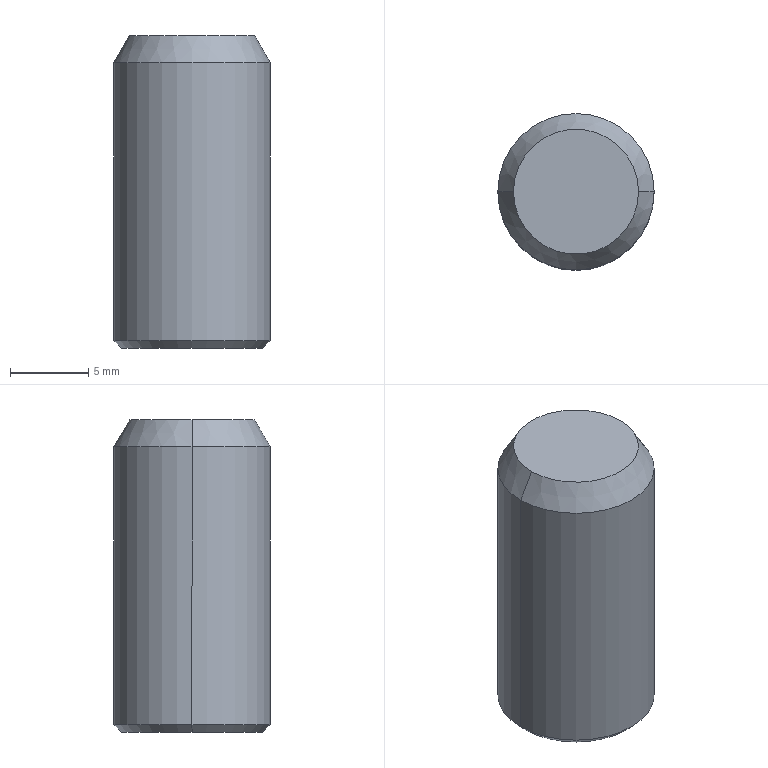Part | STEP file | Torsion pin | 1 solid | 8 faces | box 10 x 10 x 20 mm | volume 1542 mm3 | cone 4 | cylinder 2 | plane 2 | commonest cylinder face diameters 10 x2
STEP:
#1=CARTESIAN_POINT('',(0.,0.,0.));
#2=DIRECTION('',(0.,0.,1.));
#3=DIRECTION('',(1.,0.,0.));
#4=AXIS2_PLACEMENT_3D('',#1,#2,#3);
#5=CARTESIAN_POINT('',(-5.,0.,18.268));
#6=VERTEX_POINT('',#5);
#7=CARTESIAN_POINT('',(5.,0.,18.268));
#8=VERTEX_POINT('',#7);
#9=CARTESIAN_POINT('',(0.,0.,18.268));
#10=DIRECTION('',(0.,0.,-1.));
#11=DIRECTION('',(-1.,0.,0.));
#12=AXIS2_PLACEMENT_3D('',#9,#10,#11);
#13=CIRCLE('',#12,5.);
#14=CARTESIAN_POINT('',(0.,0.,20.));
#15=DIRECTION('',(0.,0.,-1.));
#16=DIRECTION('',(-1.,0.,0.));
#17=AXIS2_PLACEMENT_3D('',#14,#15,#16);
#18=CYLINDRICAL_SURFACE('',#17,5.);
#19=CARTESIAN_POINT('',(0.,1.732));
#20=DIRECTION('',(1.,0.));
#21=VECTOR('',#20,1.);
#22=LINE('',#19,#21);
#23=(GEOMETRIC_REPRESENTATION_CONTEXT(2)PARAMETRIC_REPRESENTATION_CONTEXT()REPRESENTATION_CONTEXT('',''));
#24=DEFINITIONAL_REPRESENTATION('',(#22),#23);
#25=PCURVE('',#18,#24);
#26=CARTESIAN_POINT('',(0.,0.,18.268));
#27=DIRECTION('',(0.,0.,-1.));
#28=DIRECTION('',(-1.,0.,0.));
#29=AXIS2_PLACEMENT_3D('',#26,#27,#28);
#30=CONICAL_SURFACE('',#29,5.,0.5236);
#31=CARTESIAN_POINT('',(0.,0.));
#32=DIRECTION('',(1.,0.));
#33=VECTOR('',#32,1.);
#34=LINE('',#31,#33);
#35=(GEOMETRIC_REPRESENTATION_CONTEXT(2)PARAMETRIC_REPRESENTATION_CONTEXT()REPRESENTATION_CONTEXT('',''));
#36=DEFINITIONAL_REPRESENTATION('',(#34),#35);
#37=PCURVE('',#30,#36);
#38=SURFACE_CURVE('',#13,(#25,#37),.PCURVE_S1.);
#39=EDGE_CURVE('',#6,#8,#38,.T.);
#40=ORIENTED_EDGE('',*,*,#39,.T.);
#41=CARTESIAN_POINT('',(5.,0.,0.5));
#42=VERTEX_POINT('',#41);
#43=CARTESIAN_POINT('',(5.,0.,20.));
#44=DIRECTION('',(0.,0.,-1.));
#45=VECTOR('',#44,1.);
#46=LINE('',#43,#45);
#47=CARTESIAN_POINT('',(3.142,0.));
#48=DIRECTION('',(0.,1.));
#49=VECTOR('',#48,1.);
#50=LINE('',#47,#49);
#51=(GEOMETRIC_REPRESENTATION_CONTEXT(2)PARAMETRIC_REPRESENTATION_CONTEXT()REPRESENTATION_CONTEXT('',''));
#52=DEFINITIONAL_REPRESENTATION('',(#50),#51);
#53=PCURVE('',#18,#52);
#54=CARTESIAN_POINT('',(0.,0.,20.));
#55=DIRECTION('',(0.,0.,-1.));
#56=DIRECTION('',(-1.,0.,0.));
#57=AXIS2_PLACEMENT_3D('',#54,#55,#56);
#58=CYLINDRICAL_SURFACE('',#57,5.);
#59=CARTESIAN_POINT('',(3.142,0.));
#60=DIRECTION('',(0.,1.));
#61=VECTOR('',#60,1.);
#62=LINE('',#59,#61);
#63=(GEOMETRIC_REPRESENTATION_CONTEXT(2)PARAMETRIC_REPRESENTATION_CONTEXT()REPRESENTATION_CONTEXT('',''));
#64=DEFINITIONAL_REPRESENTATION('',(#62),#63);
#65=PCURVE('',#58,#64);
#66=SURFACE_CURVE('',#46,(#53,#65),.PCURVE_S1.);
#67=EDGE_CURVE('',#8,#42,#66,.T.);
#68=ORIENTED_EDGE('',*,*,#67,.T.);
#69=CARTESIAN_POINT('',(-5.,0.,0.5));
#70=VERTEX_POINT('',#69);
#71=CARTESIAN_POINT('',(0.,0.,0.5));
#72=DIRECTION('',(0.,0.,1.));
#73=DIRECTION('',(-1.,0.,0.));
#74=AXIS2_PLACEMENT_3D('',#71,#72,#73);
#75=CIRCLE('',#74,5.);
#76=CARTESIAN_POINT('',(6.283,19.5));
#77=DIRECTION('',(-1.,0.));
#78=VECTOR('',#77,1.);
#79=LINE('',#76,#78);
#80=(GEOMETRIC_REPRESENTATION_CONTEXT(2)PARAMETRIC_REPRESENTATION_CONTEXT()REPRESENTATION_CONTEXT('',''));
#81=DEFINITIONAL_REPRESENTATION('',(#79),#80);
#82=PCURVE('',#18,#81);
#83=CARTESIAN_POINT('',(0.,0.,0.5));
#84=DIRECTION('',(0.,0.,1.));
#85=DIRECTION('',(1.,0.,0.));
#86=AXIS2_PLACEMENT_3D('',#83,#84,#85);
#87=CONICAL_SURFACE('',#86,5.,0.7854);
#88=CARTESIAN_POINT('',(-3.142,0.));
#89=DIRECTION('',(1.,0.));
#90=VECTOR('',#89,1.);
#91=LINE('',#88,#90);
#92=(GEOMETRIC_REPRESENTATION_CONTEXT(2)PARAMETRIC_REPRESENTATION_CONTEXT()REPRESENTATION_CONTEXT('',''));
#93=DEFINITIONAL_REPRESENTATION('',(#91),#92);
#94=PCURVE('',#87,#93);
#95=SURFACE_CURVE('',#75,(#82,#94),.PCURVE_S1.);
#96=EDGE_CURVE('',#42,#70,#95,.T.);
#97=ORIENTED_EDGE('',*,*,#96,.T.);
#98=CARTESIAN_POINT('',(-5.,0.,20.));
#99=DIRECTION('',(0.,0.,-1.));
#100=VECTOR('',#99,1.);
#101=LINE('',#98,#100);
#102=CARTESIAN_POINT('',(0.,0.));
#103=DIRECTION('',(0.,1.));
#104=VECTOR('',#103,1.);
#105=LINE('',#102,#104);
#106=(GEOMETRIC_REPRESENTATION_CONTEXT(2)PARAMETRIC_REPRESENTATION_CONTEXT()REPRESENTATION_CONTEXT('',''));
#107=DEFINITIONAL_REPRESENTATION('',(#105),#106);
#108=PCURVE('',#18,#107);
#109=CARTESIAN_POINT('',(6.283,0.));
#110=DIRECTION('',(0.,1.));
#111=VECTOR('',#110,1.);
#112=LINE('',#109,#111);
#113=(GEOMETRIC_REPRESENTATION_CONTEXT(2)PARAMETRIC_REPRESENTATION_CONTEXT()REPRESENTATION_CONTEXT('',''));
#114=DEFINITIONAL_REPRESENTATION('',(#112),#113);
#115=PCURVE('',#58,#114);
#116=SURFACE_CURVE('',#101,(#108,#115),.PCURVE_S1.);
#117=EDGE_CURVE('',#6,#70,#116,.T.);
#118=ORIENTED_EDGE('',*,*,#117,.F.);
#119=EDGE_LOOP('',(#40,#68,#97,#118));
#120=FACE_BOUND('',#119,.T.);
#121=ADVANCED_FACE('',(#120),#18,.T.);
#122=CARTESIAN_POINT('',(4.5,0.,0.));
#123=VERTEX_POINT('',#122);
#124=CARTESIAN_POINT('',(-4.5,0.,0.));
#125=VERTEX_POINT('',#124);
#126=CARTESIAN_POINT('',(0.,0.,0.));
#127=DIRECTION('',(0.,0.,1.));
#128=DIRECTION('',(1.,0.,0.));
#129=AXIS2_PLACEMENT_3D('',#126,#127,#128);
#130=CIRCLE('',#129,4.5);
#131=CARTESIAN_POINT('',(0.,-0.5));
#132=DIRECTION('',(1.,0.));
#133=VECTOR('',#132,1.);
#134=LINE('',#131,#133);
#135=(GEOMETRIC_REPRESENTATION_CONTEXT(2)PARAMETRIC_REPRESENTATION_CONTEXT()REPRESENTATION_CONTEXT('',''));
#136=DEFINITIONAL_REPRESENTATION('',(#134),#135);
#137=PCURVE('',#87,#136);
#138=CARTESIAN_POINT('',(0.,0.,0.));
#139=DIRECTION('',(0.,0.,1.));
#140=DIRECTION('',(1.,0.,0.));
#141=AXIS2_PLACEMENT_3D('',#138,#139,#140);
#142=PLANE('',#141);
#143=CARTESIAN_POINT('',(0.,0.));
#144=DIRECTION('',(1.,0.));
#145=AXIS2_PLACEMENT_2D('',#143,#144);
#146=CIRCLE('',#145,4.5);
#147=(GEOMETRIC_REPRESENTATION_CONTEXT(2)PARAMETRIC_REPRESENTATION_CONTEXT()REPRESENTATION_CONTEXT('',''));
#148=DEFINITIONAL_REPRESENTATION('',(#146),#147);
#149=PCURVE('',#142,#148);
#150=SURFACE_CURVE('',#130,(#137,#149),.PCURVE_S1.);
#151=EDGE_CURVE('',#123,#125,#150,.T.);
#152=ORIENTED_EDGE('',*,*,#151,.T.);
#153=CARTESIAN_POINT('',(-5.,0.,0.5));
#154=DIRECTION('',(-0.7071,0.,0.7071));
#155=VECTOR('',#154,1.);
#156=LINE('',#153,#155);
#157=CARTESIAN_POINT('',(3.142,0.));
#158=DIRECTION('',(0.,1.));
#159=VECTOR('',#158,1.);
#160=LINE('',#157,#159);
#161=(GEOMETRIC_REPRESENTATION_CONTEXT(2)PARAMETRIC_REPRESENTATION_CONTEXT()REPRESENTATION_CONTEXT('',''));
#162=DEFINITIONAL_REPRESENTATION('',(#160),#161);
#163=PCURVE('',#87,#162);
#164=CARTESIAN_POINT('',(0.,0.,0.5));
#165=DIRECTION('',(0.,0.,1.));
#166=DIRECTION('',(1.,0.,0.));
#167=AXIS2_PLACEMENT_3D('',#164,#165,#166);
#168=CONICAL_SURFACE('',#167,5.,0.7854);
#169=CARTESIAN_POINT('',(3.142,0.));
#170=DIRECTION('',(0.,1.));
#171=VECTOR('',#170,1.);
#172=LINE('',#169,#171);
#173=(GEOMETRIC_REPRESENTATION_CONTEXT(2)PARAMETRIC_REPRESENTATION_CONTEXT()REPRESENTATION_CONTEXT('',''));
#174=DEFINITIONAL_REPRESENTATION('',(#172),#173);
#175=PCURVE('',#168,#174);
#176=SURFACE_CURVE('',#156,(#163,#175),.PCURVE_S1.);
#177=EDGE_CURVE('',#125,#70,#176,.T.);
#178=ORIENTED_EDGE('',*,*,#177,.T.);
#179=ORIENTED_EDGE('',*,*,#96,.F.);
#180=CARTESIAN_POINT('',(5.,0.,0.5));
#181=DIRECTION('',(0.7071,0.,0.7071));
#182=VECTOR('',#181,1.);
#183=LINE('',#180,#182);
#184=CARTESIAN_POINT('',(0.,0.));
#185=DIRECTION('',(0.,1.));
#186=VECTOR('',#185,1.);
#187=LINE('',#184,#186);
#188=(GEOMETRIC_REPRESENTATION_CONTEXT(2)PARAMETRIC_REPRESENTATION_CONTEXT()REPRESENTATION_CONTEXT('',''));
#189=DEFINITIONAL_REPRESENTATION('',(#187),#188);
#190=PCURVE('',#87,#189);
#191=CARTESIAN_POINT('',(6.283,0.));
#192=DIRECTION('',(0.,1.));
#193=VECTOR('',#192,1.);
#194=LINE('',#191,#193);
#195=(GEOMETRIC_REPRESENTATION_CONTEXT(2)PARAMETRIC_REPRESENTATION_CONTEXT()REPRESENTATION_CONTEXT('',''));
#196=DEFINITIONAL_REPRESENTATION('',(#194),#195);
#197=PCURVE('',#168,#196);
#198=SURFACE_CURVE('',#183,(#190,#197),.PCURVE_S1.);
#199=EDGE_CURVE('',#123,#42,#198,.T.);
#200=ORIENTED_EDGE('',*,*,#199,.F.);
#201=EDGE_LOOP('',(#152,#178,#179,#200));
#202=FACE_BOUND('',#201,.T.);
#203=ADVANCED_FACE('',(#202),#87,.T.);
#204=CARTESIAN_POINT('',(-4.,0.,20.));
#205=VERTEX_POINT('',#204);
#206=CARTESIAN_POINT('',(4.,0.,20.));
#207=VERTEX_POINT('',#206);
#208=CARTESIAN_POINT('',(0.,0.,20.));
#209=DIRECTION('',(0.,0.,-1.));
#210=DIRECTION('',(-1.,0.,0.));
#211=AXIS2_PLACEMENT_3D('',#208,#209,#210);
#212=CIRCLE('',#211,4.);
#213=CARTESIAN_POINT('',(0.,-1.732));
#214=DIRECTION('',(1.,0.));
#215=VECTOR('',#214,1.);
#216=LINE('',#213,#215);
#217=(GEOMETRIC_REPRESENTATION_CONTEXT(2)PARAMETRIC_REPRESENTATION_CONTEXT()REPRESENTATION_CONTEXT('',''));
#218=DEFINITIONAL_REPRESENTATION('',(#216),#217);
#219=PCURVE('',#30,#218);
#220=CARTESIAN_POINT('',(0.,0.,20.));
#221=DIRECTION('',(0.,0.,1.));
#222=DIRECTION('',(1.,0.,0.));
#223=AXIS2_PLACEMENT_3D('',#220,#221,#222);
#224=PLANE('',#223);
#225=CARTESIAN_POINT('',(-4.,0.));
#226=CARTESIAN_POINT('',(-4.,6.928));
#227=CARTESIAN_POINT('',(2.,3.464));
#228=CARTESIAN_POINT('',(8.,0.));
#229=CARTESIAN_POINT('',(2.,-3.464));
#230=CARTESIAN_POINT('',(-4.,-6.928));
#231=CARTESIAN_POINT('',(-4.,0.));
#232=(BOUNDED_CURVE()B_SPLINE_CURVE(2,(#225,#226,#227,#228,#229,#230,#231),.UNSPECIFIED.,.T.,.F.)B_SPLINE_CURVE_WITH_KNOTS((1,2,2,2,2,1),(-2.094,0.,2.094,4.189,6.283,8.378),.UNSPECIFIED.)CURVE()GEOMETRIC_REPRESENTATION_ITEM()RATIONAL_B_SPLINE_CURVE((1.,0.5,1.,0.5,1.,0.5,1.))REPRESENTATION_ITEM(''));
#233=(GEOMETRIC_REPRESENTATION_CONTEXT(2)PARAMETRIC_REPRESENTATION_CONTEXT()REPRESENTATION_CONTEXT('',''));
#234=DEFINITIONAL_REPRESENTATION('',(#232),#233);
#235=PCURVE('',#224,#234);
#236=SURFACE_CURVE('',#212,(#219,#235),.PCURVE_S1.);
#237=EDGE_CURVE('',#205,#207,#236,.T.);
#238=ORIENTED_EDGE('',*,*,#237,.T.);
#239=CARTESIAN_POINT('',(5.,0.,18.268));
#240=DIRECTION('',(0.5,0.,-0.866));
#241=VECTOR('',#240,1.);
#242=LINE('',#239,#241);
#243=CARTESIAN_POINT('',(3.142,0.));
#244=DIRECTION('',(0.,1.));
#245=VECTOR('',#244,1.);
#246=LINE('',#243,#245);
#247=(GEOMETRIC_REPRESENTATION_CONTEXT(2)PARAMETRIC_REPRESENTATION_CONTEXT()REPRESENTATION_CONTEXT('',''));
#248=DEFINITIONAL_REPRESENTATION('',(#246),#247);
#249=PCURVE('',#30,#248);
#250=CARTESIAN_POINT('',(0.,0.,18.268));
#251=DIRECTION('',(0.,0.,-1.));
#252=DIRECTION('',(-1.,0.,0.));
#253=AXIS2_PLACEMENT_3D('',#250,#251,#252);
#254=CONICAL_SURFACE('',#253,5.,0.5236);
#255=CARTESIAN_POINT('',(3.142,0.));
#256=DIRECTION('',(0.,1.));
#257=VECTOR('',#256,1.);
#258=LINE('',#255,#257);
#259=(GEOMETRIC_REPRESENTATION_CONTEXT(2)PARAMETRIC_REPRESENTATION_CONTEXT()REPRESENTATION_CONTEXT('',''));
#260=DEFINITIONAL_REPRESENTATION('',(#258),#259);
#261=PCURVE('',#254,#260);
#262=SURFACE_CURVE('',#242,(#249,#261),.PCURVE_S1.);
#263=EDGE_CURVE('',#207,#8,#262,.T.);
#264=ORIENTED_EDGE('',*,*,#263,.T.);
#265=ORIENTED_EDGE('',*,*,#39,.F.);
#266=CARTESIAN_POINT('',(-5.,0.,18.268));
#267=DIRECTION('',(-0.5,0.,-0.866));
#268=VECTOR('',#267,1.);
#269=LINE('',#266,#268);
#270=CARTESIAN_POINT('',(0.,0.));
#271=DIRECTION('',(0.,1.));
#272=VECTOR('',#271,1.);
#273=LINE('',#270,#272);
#274=(GEOMETRIC_REPRESENTATION_CONTEXT(2)PARAMETRIC_REPRESENTATION_CONTEXT()REPRESENTATION_CONTEXT('',''));
#275=DEFINITIONAL_REPRESENTATION('',(#273),#274);
#276=PCURVE('',#30,#275);
#277=CARTESIAN_POINT('',(6.283,0.));
#278=DIRECTION('',(0.,1.));
#279=VECTOR('',#278,1.);
#280=LINE('',#277,#279);
#281=(GEOMETRIC_REPRESENTATION_CONTEXT(2)PARAMETRIC_REPRESENTATION_CONTEXT()REPRESENTATION_CONTEXT('',''));
#282=DEFINITIONAL_REPRESENTATION('',(#280),#281);
#283=PCURVE('',#254,#282);
#284=SURFACE_CURVE('',#269,(#276,#283),.PCURVE_S1.);
#285=EDGE_CURVE('',#205,#6,#284,.T.);
#286=ORIENTED_EDGE('',*,*,#285,.F.);
#287=EDGE_LOOP('',(#238,#264,#265,#286));
#288=FACE_BOUND('',#287,.T.);
#289=ADVANCED_FACE('',(#288),#30,.T.);
#290=ORIENTED_EDGE('',*,*,#67,.F.);
#291=CARTESIAN_POINT('',(0.,0.,18.268));
#292=DIRECTION('',(0.,0.,-1.));
#293=DIRECTION('',(-1.,0.,0.));
#294=AXIS2_PLACEMENT_3D('',#291,#292,#293);
#295=CIRCLE('',#294,5.);
#296=CARTESIAN_POINT('',(0.,1.732));
#297=DIRECTION('',(1.,0.));
#298=VECTOR('',#297,1.);
#299=LINE('',#296,#298);
#300=(GEOMETRIC_REPRESENTATION_CONTEXT(2)PARAMETRIC_REPRESENTATION_CONTEXT()REPRESENTATION_CONTEXT('',''));
#301=DEFINITIONAL_REPRESENTATION('',(#299),#300);
#302=PCURVE('',#58,#301);
#303=CARTESIAN_POINT('',(0.,0.));
#304=DIRECTION('',(1.,0.));
#305=VECTOR('',#304,1.);
#306=LINE('',#303,#305);
#307=(GEOMETRIC_REPRESENTATION_CONTEXT(2)PARAMETRIC_REPRESENTATION_CONTEXT()REPRESENTATION_CONTEXT('',''));
#308=DEFINITIONAL_REPRESENTATION('',(#306),#307);
#309=PCURVE('',#254,#308);
#310=SURFACE_CURVE('',#295,(#302,#309),.PCURVE_S1.);
#311=EDGE_CURVE('',#8,#6,#310,.T.);
#312=ORIENTED_EDGE('',*,*,#311,.T.);
#313=ORIENTED_EDGE('',*,*,#117,.T.);
#314=CARTESIAN_POINT('',(0.,0.,0.5));
#315=DIRECTION('',(0.,0.,1.));
#316=DIRECTION('',(-1.,0.,0.));
#317=AXIS2_PLACEMENT_3D('',#314,#315,#316);
#318=CIRCLE('',#317,5.);
#319=CARTESIAN_POINT('',(6.283,19.5));
#320=DIRECTION('',(-1.,0.));
#321=VECTOR('',#320,1.);
#322=LINE('',#319,#321);
#323=(GEOMETRIC_REPRESENTATION_CONTEXT(2)PARAMETRIC_REPRESENTATION_CONTEXT()REPRESENTATION_CONTEXT('',''));
#324=DEFINITIONAL_REPRESENTATION('',(#322),#323);
#325=PCURVE('',#58,#324);
#326=CARTESIAN_POINT('',(3.142,0.));
#327=DIRECTION('',(1.,0.));
#328=VECTOR('',#327,1.);
#329=LINE('',#326,#328);
#330=(GEOMETRIC_REPRESENTATION_CONTEXT(2)PARAMETRIC_REPRESENTATION_CONTEXT()REPRESENTATION_CONTEXT('',''));
#331=DEFINITIONAL_REPRESENTATION('',(#329),#330);
#332=PCURVE('',#168,#331);
#333=SURFACE_CURVE('',#318,(#325,#332),.PCURVE_S1.);
#334=EDGE_CURVE('',#70,#42,#333,.T.);
#335=ORIENTED_EDGE('',*,*,#334,.T.);
#336=EDGE_LOOP('',(#290,#312,#313,#335));
#337=FACE_BOUND('',#336,.T.);
#338=ADVANCED_FACE('',(#337),#58,.T.);
#339=ORIENTED_EDGE('',*,*,#177,.F.);
#340=CARTESIAN_POINT('',(0.,0.,0.));
#341=DIRECTION('',(0.,0.,1.));
#342=DIRECTION('',(1.,0.,0.));
#343=AXIS2_PLACEMENT_3D('',#340,#341,#342);
#344=CIRCLE('',#343,4.5);
#345=CARTESIAN_POINT('',(0.,-0.5));
#346=DIRECTION('',(1.,0.));
#347=VECTOR('',#346,1.);
#348=LINE('',#345,#347);
#349=(GEOMETRIC_REPRESENTATION_CONTEXT(2)PARAMETRIC_REPRESENTATION_CONTEXT()REPRESENTATION_CONTEXT('',''));
#350=DEFINITIONAL_REPRESENTATION('',(#348),#349);
#351=PCURVE('',#168,#350);
#352=CARTESIAN_POINT('',(0.,0.));
#353=DIRECTION('',(1.,0.));
#354=AXIS2_PLACEMENT_2D('',#352,#353);
#355=CIRCLE('',#354,4.5);
#356=(GEOMETRIC_REPRESENTATION_CONTEXT(2)PARAMETRIC_REPRESENTATION_CONTEXT()REPRESENTATION_CONTEXT('',''));
#357=DEFINITIONAL_REPRESENTATION('',(#355),#356);
#358=PCURVE('',#142,#357);
#359=SURFACE_CURVE('',#344,(#351,#358),.PCURVE_S1.);
#360=EDGE_CURVE('',#125,#123,#359,.T.);
#361=ORIENTED_EDGE('',*,*,#360,.T.);
#362=ORIENTED_EDGE('',*,*,#199,.T.);
#363=ORIENTED_EDGE('',*,*,#334,.F.);
#364=EDGE_LOOP('',(#339,#361,#362,#363));
#365=FACE_BOUND('',#364,.T.);
#366=ADVANCED_FACE('',(#365),#168,.T.);
#367=ORIENTED_EDGE('',*,*,#263,.F.);
#368=CARTESIAN_POINT('',(0.,0.,20.));
#369=DIRECTION('',(0.,0.,-1.));
#370=DIRECTION('',(-1.,0.,0.));
#371=AXIS2_PLACEMENT_3D('',#368,#369,#370);
#372=CIRCLE('',#371,4.);
#373=CARTESIAN_POINT('',(0.,-1.732));
#374=DIRECTION('',(1.,0.));
#375=VECTOR('',#374,1.);
#376=LINE('',#373,#375);
#377=(GEOMETRIC_REPRESENTATION_CONTEXT(2)PARAMETRIC_REPRESENTATION_CONTEXT()REPRESENTATION_CONTEXT('',''));
#378=DEFINITIONAL_REPRESENTATION('',(#376),#377);
#379=PCURVE('',#254,#378);
#380=CARTESIAN_POINT('',(-4.,0.));
#381=CARTESIAN_POINT('',(-4.,6.928));
#382=CARTESIAN_POINT('',(2.,3.464));
#383=CARTESIAN_POINT('',(8.,0.));
#384=CARTESIAN_POINT('',(2.,-3.464));
#385=CARTESIAN_POINT('',(-4.,-6.928));
#386=CARTESIAN_POINT('',(-4.,0.));
#387=(BOUNDED_CURVE()B_SPLINE_CURVE(2,(#380,#381,#382,#383,#384,#385,#386),.UNSPECIFIED.,.T.,.F.)B_SPLINE_CURVE_WITH_KNOTS((1,2,2,2,2,1),(-2.094,0.,2.094,4.189,6.283,8.378),.UNSPECIFIED.)CURVE()GEOMETRIC_REPRESENTATION_ITEM()RATIONAL_B_SPLINE_CURVE((1.,0.5,1.,0.5,1.,0.5,1.))REPRESENTATION_ITEM(''));
#388=(GEOMETRIC_REPRESENTATION_CONTEXT(2)PARAMETRIC_REPRESENTATION_CONTEXT()REPRESENTATION_CONTEXT('',''));
#389=DEFINITIONAL_REPRESENTATION('',(#387),#388);
#390=PCURVE('',#224,#389);
#391=SURFACE_CURVE('',#372,(#379,#390),.PCURVE_S1.);
#392=EDGE_CURVE('',#207,#205,#391,.T.);
#393=ORIENTED_EDGE('',*,*,#392,.T.);
#394=ORIENTED_EDGE('',*,*,#285,.T.);
#395=ORIENTED_EDGE('',*,*,#311,.F.);
#396=EDGE_LOOP('',(#367,#393,#394,#395));
#397=FACE_BOUND('',#396,.T.);
#398=ADVANCED_FACE('',(#397),#254,.T.);
#399=ORIENTED_EDGE('',*,*,#151,.F.);
#400=ORIENTED_EDGE('',*,*,#360,.F.);
#401=EDGE_LOOP('',(#399,#400));
#402=FACE_BOUND('',#401,.T.);
#403=ADVANCED_FACE('',(#402),#142,.F.);
#404=ORIENTED_EDGE('',*,*,#237,.F.);
#405=ORIENTED_EDGE('',*,*,#392,.F.);
#406=EDGE_LOOP('',(#404,#405));
#407=FACE_BOUND('',#406,.T.);
#408=ADVANCED_FACE('',(#407),#224,.T.);
#409=CLOSED_SHELL('',(#121,#203,#289,#338,#366,#398,#403,#408));
#410=MANIFOLD_SOLID_BREP('',#409);
#411=(LENGTH_UNIT()NAMED_UNIT(*)SI_UNIT(.MILLI.,.METRE.));
#412=UNCERTAINTY_MEASURE_WITH_UNIT(LENGTH_MEASURE(0.0000001),#411,'','');
#413=(NAMED_UNIT(*)PLANE_ANGLE_UNIT()SI_UNIT($,.RADIAN.));
#414=(NAMED_UNIT(*)SI_UNIT($,.STERADIAN.)SOLID_ANGLE_UNIT());
#415=(GEOMETRIC_REPRESENTATION_CONTEXT(3)GLOBAL_UNCERTAINTY_ASSIGNED_CONTEXT((#412))GLOBAL_UNIT_ASSIGNED_CONTEXT((#411,#413,#414))REPRESENTATION_CONTEXT('',''));
#416=ADVANCED_BREP_SHAPE_REPRESENTATION('',(#4,#410),#415);